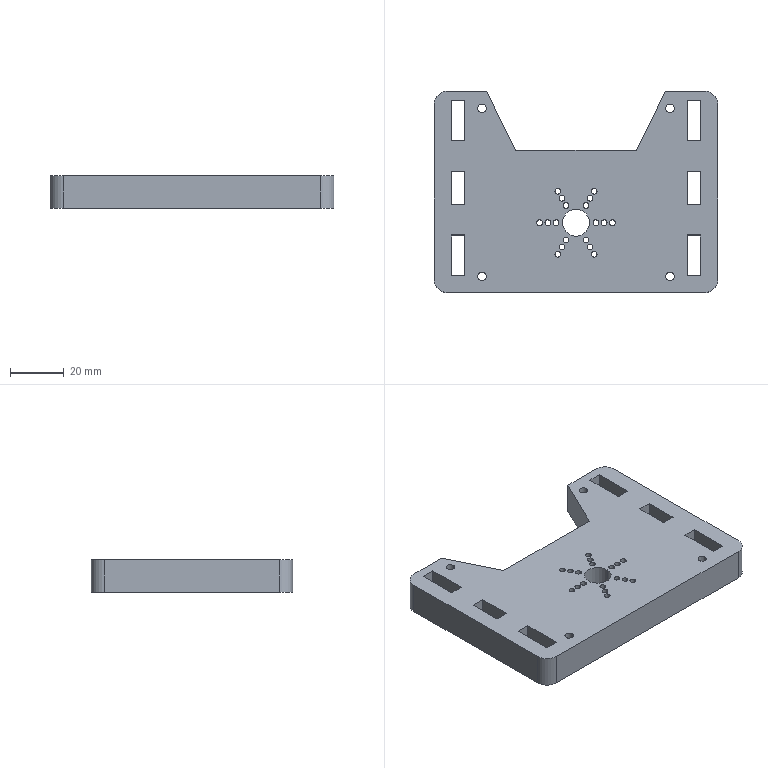Part | SolidWorks | features Extrusion 1 | 1 solid | 84 faces | box 105.6 x 75 x 12 mm | volume 72869 mm3 | cylinder 50 | plane 34 | commonest cylinder face diameters 2.15 x36 3.15 x8 10 x6